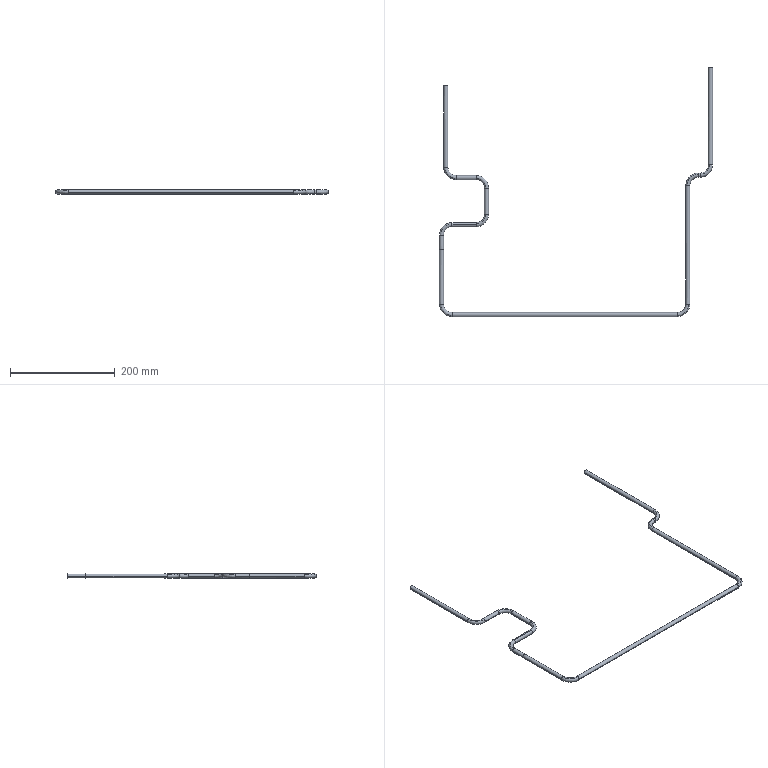Part | 1 solid | 40 faces | box 521.696 x 476.176 x 8 mm | volume 76293 mm3 | cylinder 20 | torus 16 | plane 4 | commonest cylinder face diameters 8 x20